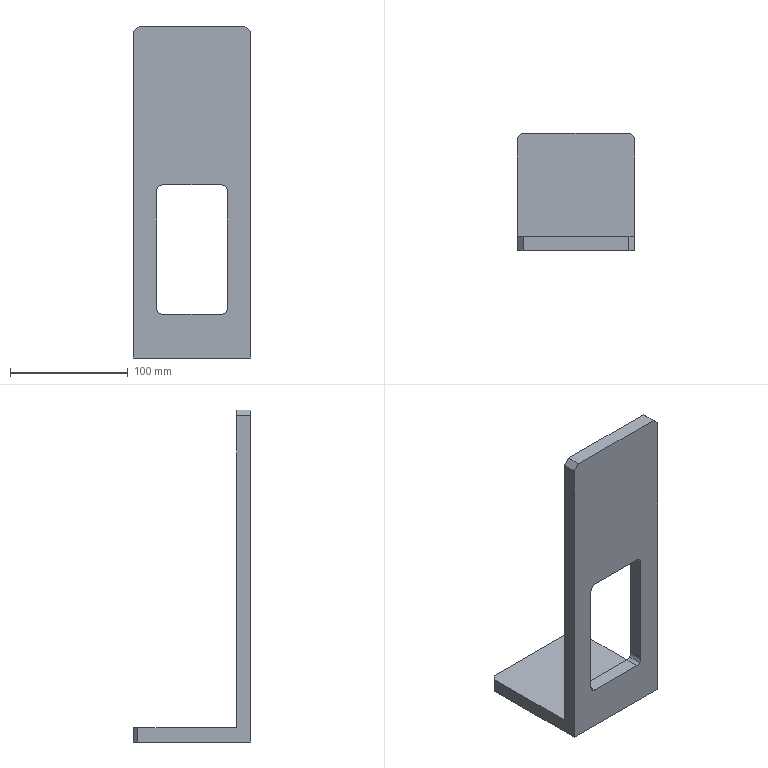Part | STEP file | ASND-0110-Body 1-27 | 1 solid | 24 faces | box 100 x 100 x 282 mm | volume 364566 mm3 | plane 16 | cylinder 8 | commonest cylinder face diameters 10 x8